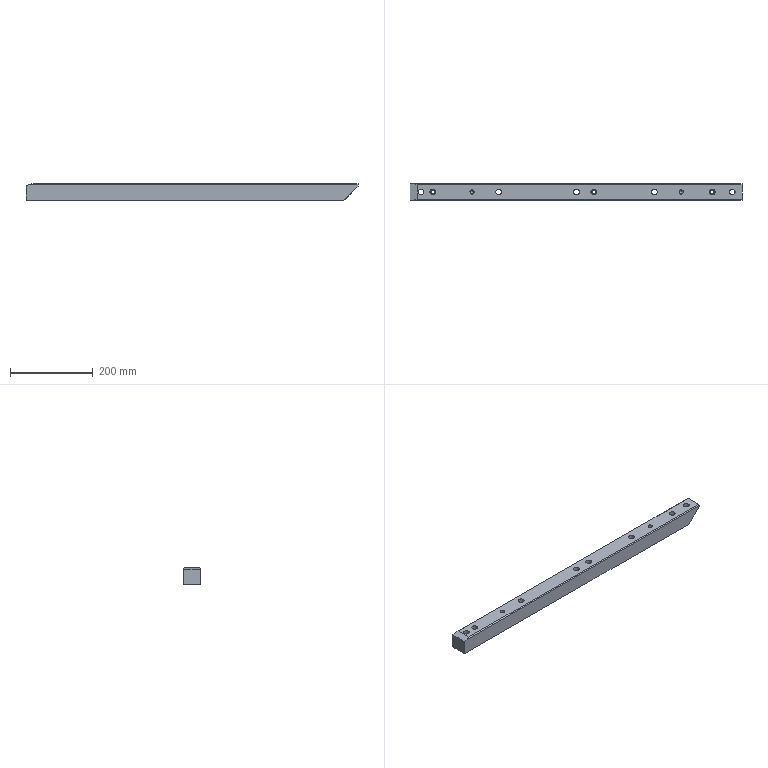Part | NX | features 22 2 | 1 solid | 47 faces | box 802 x 40 x 40 mm | volume 1188494 mm3 | cylinder 24 | plane 19 | cone 4 | commonest cylinder face diameters 14 x8 6 x6 9 x3 25 x3 6.8 x2 10.3 x2
STEP:
#1=CARTESIAN_POINT('',(3434.4,-12.,-43.5));
#2=VERTEX_POINT('',#1);
#3=CARTESIAN_POINT('',(3431.,-12.,-43.5));
#4=DIRECTION('',(0.,0.,1.));
#5=DIRECTION('',(1.,0.,0.));
#6=AXIS2_PLACEMENT_3D('',#3,#4,#5);
#7=CIRCLE('',#6,3.4);
#8=EDGE_CURVE('',#2,#2,#7,.T.);
#9=ORIENTED_EDGE('',*,*,#8,.T.);
#10=EDGE_LOOP('',(#9));
#11=FACE_BOUND('',#10,.T.);
#12=CARTESIAN_POINT('',(3224.306,0.,-43.5));
#13=VERTEX_POINT('',#12);
#14=CARTESIAN_POINT('',(3217.306,0.,-43.5));
#15=DIRECTION('',(0.,0.,-1.));
#16=DIRECTION('',(1.,0.,0.));
#17=AXIS2_PLACEMENT_3D('',#14,#15,#16);
#18=CIRCLE('',#17,7.);
#19=EDGE_CURVE('',#13,#13,#18,.T.);
#20=ORIENTED_EDGE('',*,*,#19,.F.);
#21=EDGE_LOOP('',(#20));
#22=FACE_BOUND('',#21,.T.);
#23=CARTESIAN_POINT('',(2848.306,0.,-43.5));
#24=VERTEX_POINT('',#23);
#25=CARTESIAN_POINT('',(2841.306,0.,-43.5));
#26=DIRECTION('',(0.,0.,-1.));
#27=DIRECTION('',(1.,0.,0.));
#28=AXIS2_PLACEMENT_3D('',#25,#26,#27);
#29=CIRCLE('',#28,7.);
#30=EDGE_CURVE('',#24,#24,#29,.T.);
#31=ORIENTED_EDGE('',*,*,#30,.F.);
#32=EDGE_LOOP('',(#31));
#33=FACE_BOUND('',#32,.T.);
#34=CARTESIAN_POINT('',(3412.306,0.,-43.5));
#35=VERTEX_POINT('',#34);
#36=CARTESIAN_POINT('',(3405.306,0.,-43.5));
#37=DIRECTION('',(0.,0.,-1.));
#38=DIRECTION('',(1.,0.,0.));
#39=AXIS2_PLACEMENT_3D('',#36,#37,#38);
#40=CIRCLE('',#39,7.);
#41=EDGE_CURVE('',#35,#35,#40,.T.);
#42=ORIENTED_EDGE('',*,*,#41,.F.);
#43=EDGE_LOOP('',(#42));
#44=FACE_BOUND('',#43,.T.);
#45=CARTESIAN_POINT('',(3547.701,-11.,-43.5));
#46=VERTEX_POINT('',#45);
#47=CARTESIAN_POINT('',(3542.299,-11.,-43.5));
#48=VERTEX_POINT('',#47);
#49=CARTESIAN_POINT('',(3545.,-11.,-43.5));
#50=DIRECTION('',(-1.,0.,0.));
#51=VECTOR('',#50,1000.);
#52=LINE('',#49,#51);
#53=EDGE_CURVE('',#46,#48,#52,.T.);
#54=ORIENTED_EDGE('',*,*,#53,.F.);
#55=CARTESIAN_POINT('',(3552.847,-9.73,-43.5));
#56=VERTEX_POINT('',#55);
#57=CARTESIAN_POINT('',(3549.937,-9.,-43.5));
#58=DIRECTION('',(0.,0.,-1.));
#59=DIRECTION('',(1.,0.,0.));
#60=AXIS2_PLACEMENT_3D('',#57,#58,#59);
#61=CIRCLE('',#60,3.);
#62=EDGE_CURVE('',#56,#46,#61,.T.);
#63=ORIENTED_EDGE('',*,*,#62,.F.);
#64=CARTESIAN_POINT('',(3537.153,-9.73,-43.5));
#65=VERTEX_POINT('',#64);
#66=CARTESIAN_POINT('',(3545.,0.,-43.5));
#67=DIRECTION('',(0.,0.,-1.));
#68=DIRECTION('',(1.,0.,0.));
#69=AXIS2_PLACEMENT_3D('',#66,#67,#68);
#70=CIRCLE('',#69,12.5);
#71=EDGE_CURVE('',#65,#56,#70,.T.);
#72=ORIENTED_EDGE('',*,*,#71,.F.);
#73=CARTESIAN_POINT('',(3540.063,-9.,-43.5));
#74=DIRECTION('',(0.,0.,-1.));
#75=DIRECTION('',(1.,0.,0.));
#76=AXIS2_PLACEMENT_3D('',#73,#74,#75);
#77=CIRCLE('',#76,3.);
#78=EDGE_CURVE('',#48,#65,#77,.T.);
#79=ORIENTED_EDGE('',*,*,#78,.F.);
#80=EDGE_LOOP('',(#54,#63,#72,#79));
#81=FACE_BOUND('',#80,.T.);
#82=CARTESIAN_POINT('',(2872.701,-11.,-43.5));
#83=VERTEX_POINT('',#82);
#84=CARTESIAN_POINT('',(2867.299,-11.,-43.5));
#85=VERTEX_POINT('',#84);
#86=CARTESIAN_POINT('',(2870.,-11.,-43.5));
#87=DIRECTION('',(-1.,0.,0.));
#88=VECTOR('',#87,1000.);
#89=LINE('',#86,#88);
#90=EDGE_CURVE('',#83,#85,#89,.T.);
#91=ORIENTED_EDGE('',*,*,#90,.F.);
#92=CARTESIAN_POINT('',(2877.847,-9.73,-43.5));
#93=VERTEX_POINT('',#92);
#94=CARTESIAN_POINT('',(2874.937,-9.,-43.5));
#95=DIRECTION('',(0.,0.,-1.));
#96=DIRECTION('',(0.9659,0.2588,0.));
#97=AXIS2_PLACEMENT_3D('',#94,#95,#96);
#98=CIRCLE('',#97,3.);
#99=EDGE_CURVE('',#93,#83,#98,.T.);
#100=ORIENTED_EDGE('',*,*,#99,.F.);
#101=CARTESIAN_POINT('',(2862.153,-9.73,-43.5));
#102=VERTEX_POINT('',#101);
#103=CARTESIAN_POINT('',(2870.,0.,-43.5));
#104=DIRECTION('',(0.,0.,1.));
#105=DIRECTION('',(0.9659,0.2588,0.));
#106=AXIS2_PLACEMENT_3D('',#103,#104,#105);
#107=CIRCLE('',#106,12.5);
#108=EDGE_CURVE('',#93,#102,#107,.T.);
#109=ORIENTED_EDGE('',*,*,#108,.T.);
#110=CARTESIAN_POINT('',(2865.063,-9.,-43.5));
#111=DIRECTION('',(0.,0.,-1.));
#112=DIRECTION('',(0.9659,0.2588,0.));
#113=AXIS2_PLACEMENT_3D('',#110,#111,#112);
#114=CIRCLE('',#113,3.);
#115=EDGE_CURVE('',#85,#102,#114,.T.);
#116=ORIENTED_EDGE('',*,*,#115,.F.);
#117=EDGE_LOOP('',(#91,#100,#109,#116));
#118=FACE_BOUND('',#117,.T.);
#119=CARTESIAN_POINT('',(3583.,20.,-43.5));
#120=VERTEX_POINT('',#119);
#121=CARTESIAN_POINT('',(2815.,20.,-43.5));
#122=VERTEX_POINT('',#121);
#123=CARTESIAN_POINT('',(2860.,20.,-43.5));
#124=DIRECTION('',(-1.,0.,0.));
#125=VECTOR('',#124,1000.);
#126=LINE('',#123,#125);
#127=EDGE_CURVE('',#120,#122,#126,.T.);
#128=ORIENTED_EDGE('',*,*,#127,.F.);
#129=CARTESIAN_POINT('',(3583.,-20.,-43.5));
#130=VERTEX_POINT('',#129);
#131=CARTESIAN_POINT('',(3583.,0.,-43.5));
#132=DIRECTION('',(0.,-1.,0.));
#133=VECTOR('',#132,1000.);
#134=LINE('',#131,#133);
#135=EDGE_CURVE('',#120,#130,#134,.T.);
#136=ORIENTED_EDGE('',*,*,#135,.T.);
#137=CARTESIAN_POINT('',(2815.,-20.,-43.5));
#138=VERTEX_POINT('',#137);
#139=CARTESIAN_POINT('',(2860.,-20.,-43.5));
#140=DIRECTION('',(1.,0.,0.));
#141=VECTOR('',#140,1000.);
#142=LINE('',#139,#141);
#143=EDGE_CURVE('',#138,#130,#142,.T.);
#144=ORIENTED_EDGE('',*,*,#143,.F.);
#145=CARTESIAN_POINT('',(2815.,0.,-43.5));
#146=DIRECTION('',(0.,-1.,0.));
#147=VECTOR('',#146,1000.);
#148=LINE('',#145,#147);
#149=EDGE_CURVE('',#122,#138,#148,.T.);
#150=ORIENTED_EDGE('',*,*,#149,.F.);
#151=EDGE_LOOP('',(#128,#136,#144,#150));
#152=FACE_BOUND('',#151,.T.);
#153=CARTESIAN_POINT('',(3036.306,0.,-43.5));
#154=VERTEX_POINT('',#153);
#155=CARTESIAN_POINT('',(3029.306,0.,-43.5));
#156=DIRECTION('',(0.,0.,-1.));
#157=DIRECTION('',(1.,0.,0.));
#158=AXIS2_PLACEMENT_3D('',#155,#156,#157);
#159=CIRCLE('',#158,7.);
#160=EDGE_CURVE('',#154,#154,#159,.T.);
#161=ORIENTED_EDGE('',*,*,#160,.F.);
#162=EDGE_LOOP('',(#161));
#163=FACE_BOUND('',#162,.T.);
#164=CARTESIAN_POINT('',(3251.153,-9.73,-43.5));
#165=VERTEX_POINT('',#164);
#166=CARTESIAN_POINT('',(3266.847,-9.73,-43.5));
#167=VERTEX_POINT('',#166);
#168=CARTESIAN_POINT('',(3259.,0.,-43.5));
#169=DIRECTION('',(0.,0.,-1.));
#170=DIRECTION('',(1.,0.,0.));
#171=AXIS2_PLACEMENT_3D('',#168,#169,#170);
#172=CIRCLE('',#171,12.5);
#173=EDGE_CURVE('',#165,#167,#172,.T.);
#174=ORIENTED_EDGE('',*,*,#173,.F.);
#175=CARTESIAN_POINT('',(3256.299,-11.,-43.5));
#176=VERTEX_POINT('',#175);
#177=CARTESIAN_POINT('',(3254.063,-9.,-43.5));
#178=DIRECTION('',(0.,0.,1.));
#179=DIRECTION('',(1.,0.,0.));
#180=AXIS2_PLACEMENT_3D('',#177,#178,#179);
#181=CIRCLE('',#180,3.);
#182=EDGE_CURVE('',#165,#176,#181,.T.);
#183=ORIENTED_EDGE('',*,*,#182,.T.);
#184=CARTESIAN_POINT('',(3261.701,-11.,-43.5));
#185=VERTEX_POINT('',#184);
#186=CARTESIAN_POINT('',(2534.879,-11.,-43.5));
#187=DIRECTION('',(1.,0.,0.));
#188=VECTOR('',#187,1000.);
#189=LINE('',#186,#188);
#190=EDGE_CURVE('',#176,#185,#189,.T.);
#191=ORIENTED_EDGE('',*,*,#190,.T.);
#192=CARTESIAN_POINT('',(3263.937,-9.,-43.5));
#193=DIRECTION('',(0.,0.,1.));
#194=DIRECTION('',(1.,0.,0.));
#195=AXIS2_PLACEMENT_3D('',#192,#193,#194);
#196=CIRCLE('',#195,3.);
#197=EDGE_CURVE('',#185,#167,#196,.T.);
#198=ORIENTED_EDGE('',*,*,#197,.T.);
#199=EDGE_LOOP('',(#174,#183,#191,#198));
#200=FACE_BOUND('',#199,.T.);
#201=CARTESIAN_POINT('',(3434.4,12.,-43.5));
#202=VERTEX_POINT('',#201);
#203=CARTESIAN_POINT('',(3431.,12.,-43.5));
#204=DIRECTION('',(0.,0.,1.));
#205=DIRECTION('',(1.,0.,0.));
#206=AXIS2_PLACEMENT_3D('',#203,#204,#205);
#207=CIRCLE('',#206,3.4);
#208=EDGE_CURVE('',#202,#202,#207,.T.);
#209=ORIENTED_EDGE('',*,*,#208,.T.);
#210=EDGE_LOOP('',(#209));
#211=FACE_BOUND('',#210,.T.);
#212=CARTESIAN_POINT('',(2544.879,0.,-43.5));
#213=DIRECTION('',(0.,0.,1.));
#214=DIRECTION('',(-1.,0.,0.));
#215=AXIS2_PLACEMENT_3D('',#212,#213,#214);
#216=PLANE('',#215);
#217=ADVANCED_FACE('',(#11,#22,#33,#44,#81,#118,#152,#163,#200,#211),#216,.F.);
#218=CARTESIAN_POINT('',(3263.229,1.539,-28.5));
#219=VERTEX_POINT('',#218);
#220=CARTESIAN_POINT('',(3259.,0.,-28.5));
#221=DIRECTION('',(0.,0.,1.));
#222=DIRECTION('',(0.9397,0.342,0.));
#223=AXIS2_PLACEMENT_3D('',#220,#221,#222);
#224=CIRCLE('',#223,4.5);
#225=EDGE_CURVE('',#219,#219,#224,.T.);
#226=ORIENTED_EDGE('',*,*,#225,.F.);
#227=EDGE_LOOP('',(#226));
#228=FACE_BOUND('',#227,.T.);
#229=CARTESIAN_POINT('',(3263.5,0.,-15.5));
#230=VERTEX_POINT('',#229);
#231=CARTESIAN_POINT('',(3259.,0.,-15.5));
#232=DIRECTION('',(0.,0.,1.));
#233=DIRECTION('',(1.,0.,0.));
#234=AXIS2_PLACEMENT_3D('',#231,#232,#233);
#235=CIRCLE('',#234,4.5);
#236=EDGE_CURVE('',#230,#230,#235,.T.);
#237=ORIENTED_EDGE('',*,*,#236,.T.);
#238=EDGE_LOOP('',(#237));
#239=FACE_BOUND('',#238,.T.);
#240=CARTESIAN_POINT('',(3259.,0.,49.9));
#241=DIRECTION('',(0.,0.,-1.));
#242=DIRECTION('',(0.342,-0.9397,0.));
#243=AXIS2_PLACEMENT_3D('',#240,#241,#242);
#244=CYLINDRICAL_SURFACE('',#243,4.5);
#245=ADVANCED_FACE('',(#228,#239),#244,.F.);
#246=ORIENTED_EDGE('',*,*,#225,.T.);
#247=EDGE_LOOP('',(#246));
#248=FACE_BOUND('',#247,.T.);
#249=CARTESIAN_POINT('',(3256.299,-11.,-28.5));
#250=VERTEX_POINT('',#249);
#251=CARTESIAN_POINT('',(3251.153,-9.73,-28.5));
#252=VERTEX_POINT('',#251);
#253=CARTESIAN_POINT('',(3254.063,-9.,-28.5));
#254=DIRECTION('',(0.,0.,-1.));
#255=DIRECTION('',(0.9397,-0.342,0.));
#256=AXIS2_PLACEMENT_3D('',#253,#254,#255);
#257=CIRCLE('',#256,3.);
#258=EDGE_CURVE('',#250,#252,#257,.T.);
#259=ORIENTED_EDGE('',*,*,#258,.T.);
#260=CARTESIAN_POINT('',(3266.847,-9.73,-28.5));
#261=VERTEX_POINT('',#260);
#262=CARTESIAN_POINT('',(3259.,0.,-28.5));
#263=DIRECTION('',(0.,0.,-1.));
#264=DIRECTION('',(0.,1.,0.));
#265=AXIS2_PLACEMENT_3D('',#262,#263,#264);
#266=CIRCLE('',#265,12.5);
#267=EDGE_CURVE('',#252,#261,#266,.T.);
#268=ORIENTED_EDGE('',*,*,#267,.T.);
#269=CARTESIAN_POINT('',(3261.701,-11.,-28.5));
#270=VERTEX_POINT('',#269);
#271=CARTESIAN_POINT('',(3263.937,-9.,-28.5));
#272=DIRECTION('',(0.,0.,1.));
#273=DIRECTION('',(-0.9397,-0.342,0.));
#274=AXIS2_PLACEMENT_3D('',#271,#272,#273);
#275=CIRCLE('',#274,3.);
#276=EDGE_CURVE('',#270,#261,#275,.T.);
#277=ORIENTED_EDGE('',*,*,#276,.F.);
#278=CARTESIAN_POINT('',(3259.,-11.,-28.5));
#279=DIRECTION('',(-1.,0.,0.));
#280=VECTOR('',#279,1000.);
#281=LINE('',#278,#280);
#282=EDGE_CURVE('',#270,#250,#281,.T.);
#283=ORIENTED_EDGE('',*,*,#282,.T.);
#284=EDGE_LOOP('',(#259,#268,#277,#283));
#285=FACE_BOUND('',#284,.T.);
#286=CARTESIAN_POINT('',(3259.,0.,-28.5));
#287=DIRECTION('',(0.,0.,1.));
#288=DIRECTION('',(0.,-1.,0.));
#289=AXIS2_PLACEMENT_3D('',#286,#287,#288);
#290=PLANE('',#289);
#291=ADVANCED_FACE('',(#248,#285),#290,.F.);
#292=ORIENTED_EDGE('',*,*,#282,.F.);
#293=CARTESIAN_POINT('',(3261.701,-11.,-41.5));
#294=DIRECTION('',(0.,0.,1.));
#295=VECTOR('',#294,1000.);
#296=LINE('',#293,#295);
#297=EDGE_CURVE('',#185,#270,#296,.T.);
#298=ORIENTED_EDGE('',*,*,#297,.F.);
#299=ORIENTED_EDGE('',*,*,#190,.F.);
#300=CARTESIAN_POINT('',(3256.299,-11.,-41.5));
#301=DIRECTION('',(0.,0.,1.));
#302=VECTOR('',#301,1000.);
#303=LINE('',#300,#302);
#304=EDGE_CURVE('',#176,#250,#303,.T.);
#305=ORIENTED_EDGE('',*,*,#304,.T.);
#306=EDGE_LOOP('',(#292,#298,#299,#305));
#307=FACE_BOUND('',#306,.T.);
#308=CARTESIAN_POINT('',(3259.,-11.,-126.5));
#309=DIRECTION('',(0.,1.,0.));
#310=DIRECTION('',(0.,0.,-1.));
#311=AXIS2_PLACEMENT_3D('',#308,#309,#310);
#312=PLANE('',#311);
#313=ADVANCED_FACE('',(#307),#312,.T.);
#314=CARTESIAN_POINT('',(3266.847,-9.73,-34.));
#315=DIRECTION('',(0.,0.,-1.));
#316=VECTOR('',#315,1000.);
#317=LINE('',#314,#316);
#318=EDGE_CURVE('',#261,#167,#317,.T.);
#319=ORIENTED_EDGE('',*,*,#318,.F.);
#320=ORIENTED_EDGE('',*,*,#267,.F.);
#321=CARTESIAN_POINT('',(3251.153,-9.73,-34.));
#322=DIRECTION('',(0.,0.,-1.));
#323=VECTOR('',#322,1000.);
#324=LINE('',#321,#323);
#325=EDGE_CURVE('',#252,#165,#324,.T.);
#326=ORIENTED_EDGE('',*,*,#325,.T.);
#327=ORIENTED_EDGE('',*,*,#173,.T.);
#328=EDGE_LOOP('',(#319,#320,#326,#327));
#329=FACE_BOUND('',#328,.T.);
#330=CARTESIAN_POINT('',(3259.,0.,-96.5));
#331=DIRECTION('',(0.,0.,-1.));
#332=DIRECTION('',(0.,1.,0.));
#333=AXIS2_PLACEMENT_3D('',#330,#331,#332);
#334=CYLINDRICAL_SURFACE('',#333,12.5);
#335=ADVANCED_FACE('',(#329),#334,.F.);
#336=ORIENTED_EDGE('',*,*,#318,.T.);
#337=ORIENTED_EDGE('',*,*,#197,.F.);
#338=ORIENTED_EDGE('',*,*,#297,.T.);
#339=ORIENTED_EDGE('',*,*,#276,.T.);
#340=EDGE_LOOP('',(#336,#337,#338,#339));
#341=FACE_BOUND('',#340,.T.);
#342=CARTESIAN_POINT('',(3263.937,-9.,-41.5));
#343=DIRECTION('',(0.,0.,1.));
#344=DIRECTION('',(-0.9397,-0.342,0.));
#345=AXIS2_PLACEMENT_3D('',#342,#343,#344);
#346=CYLINDRICAL_SURFACE('',#345,3.);
#347=ADVANCED_FACE('',(#341),#346,.F.);
#348=ORIENTED_EDGE('',*,*,#325,.F.);
#349=ORIENTED_EDGE('',*,*,#258,.F.);
#350=ORIENTED_EDGE('',*,*,#304,.F.);
#351=ORIENTED_EDGE('',*,*,#182,.F.);
#352=EDGE_LOOP('',(#348,#349,#350,#351));
#353=FACE_BOUND('',#352,.T.);
#354=CARTESIAN_POINT('',(3254.063,-9.,-41.5));
#355=DIRECTION('',(0.,0.,1.));
#356=DIRECTION('',(0.9397,-0.342,0.));
#357=AXIS2_PLACEMENT_3D('',#354,#355,#356);
#358=CYLINDRICAL_SURFACE('',#357,3.);
#359=ADVANCED_FACE('',(#353),#358,.F.);
#360=CARTESIAN_POINT('',(3266.,0.,-15.5));
#361=VERTEX_POINT('',#360);
#362=CARTESIAN_POINT('',(3259.,0.,-15.5));
#363=DIRECTION('',(0.,0.,1.));
#364=DIRECTION('',(1.,0.,0.));
#365=AXIS2_PLACEMENT_3D('',#362,#363,#364);
#366=CIRCLE('',#365,7.);
#367=EDGE_CURVE('',#361,#361,#366,.T.);
#368=ORIENTED_EDGE('',*,*,#367,.T.);
#369=EDGE_LOOP('',(#368));
#370=FACE_BOUND('',#369,.T.);
#371=ORIENTED_EDGE('',*,*,#236,.F.);
#372=EDGE_LOOP('',(#371));
#373=FACE_BOUND('',#372,.T.);
#374=CARTESIAN_POINT('',(3377.182,268.173,-15.5));
#375=DIRECTION('',(0.,0.,1.));
#376=DIRECTION('',(-0.9397,-0.342,0.));
#377=AXIS2_PLACEMENT_3D('',#374,#375,#376);
#378=PLANE('',#377);
#379=ADVANCED_FACE('',(#370,#373),#378,.T.);
#380=CARTESIAN_POINT('',(3266.,0.,-3.5));
#381=VERTEX_POINT('',#380);
#382=CARTESIAN_POINT('',(3259.,0.,-3.5));
#383=DIRECTION('',(0.,0.,1.));
#384=DIRECTION('',(1.,0.,0.));
#385=AXIS2_PLACEMENT_3D('',#382,#383,#384);
#386=CIRCLE('',#385,7.);
#387=EDGE_CURVE('',#381,#381,#386,.T.);
#388=ORIENTED_EDGE('',*,*,#387,.T.);
#389=EDGE_LOOP('',(#388));
#390=FACE_BOUND('',#389,.T.);
#391=ORIENTED_EDGE('',*,*,#367,.F.);
#392=EDGE_LOOP('',(#391));
#393=FACE_BOUND('',#392,.T.);
#394=CARTESIAN_POINT('',(3259.,0.,-9.5));
#395=DIRECTION('',(0.,0.,1.));
#396=DIRECTION('',(-0.9397,-0.342,0.));
#397=AXIS2_PLACEMENT_3D('',#394,#395,#396);
#398=CYLINDRICAL_SURFACE('',#397,7.);
#399=ADVANCED_FACE('',(#390,#393),#398,.F.);
#400=CARTESIAN_POINT('',(2874.229,1.539,-28.5));
#401=VERTEX_POINT('',#400);
#402=CARTESIAN_POINT('',(2870.,0.,-28.5));
#403=DIRECTION('',(0.,0.,1.));
#404=DIRECTION('',(0.9397,0.342,0.));
#405=AXIS2_PLACEMENT_3D('',#402,#403,#404);
#406=CIRCLE('',#405,4.5);
#407=EDGE_CURVE('',#401,#401,#406,.T.);
#408=ORIENTED_EDGE('',*,*,#407,.F.);
#409=EDGE_LOOP('',(#408));
#410=FACE_BOUND('',#409,.T.);
#411=CARTESIAN_POINT('',(2874.5,0.,-15.5));
#412=VERTEX_POINT('',#411);
#413=CARTESIAN_POINT('',(2870.,0.,-15.5));
#414=DIRECTION('',(0.,0.,1.));
#415=DIRECTION('',(1.,0.,0.));
#416=AXIS2_PLACEMENT_3D('',#413,#414,#415);
#417=CIRCLE('',#416,4.5);
#418=EDGE_CURVE('',#412,#412,#417,.T.);
#419=ORIENTED_EDGE('',*,*,#418,.T.);
#420=EDGE_LOOP('',(#419));
#421=FACE_BOUND('',#420,.T.);
#422=CARTESIAN_POINT('',(2870.,0.,49.9));
#423=DIRECTION('',(0.,0.,-1.));
#424=DIRECTION('',(0.342,-0.9397,0.));
#425=AXIS2_PLACEMENT_3D('',#422,#423,#424);
#426=CYLINDRICAL_SURFACE('',#425,4.5);
#427=ADVANCED_FACE('',(#410,#421),#426,.F.);
#428=CARTESIAN_POINT('',(3545.,-4.5,-28.5));
#429=VERTEX_POINT('',#428);
#430=CARTESIAN_POINT('',(3545.,0.,-28.5));
#431=DIRECTION('',(0.,0.,1.));
#432=DIRECTION('',(0.,-1.,0.));
#433=AXIS2_PLACEMENT_3D('',#430,#431,#432);
#434=CIRCLE('',#433,4.5);
#435=EDGE_CURVE('',#429,#429,#434,.T.);
#436=ORIENTED_EDGE('',*,*,#435,.F.);
#437=EDGE_LOOP('',(#436));
#438=FACE_BOUND('',#437,.T.);
#439=CARTESIAN_POINT('',(3545.,-4.5,-15.5));
#440=VERTEX_POINT('',#439);
#441=CARTESIAN_POINT('',(3545.,0.,-15.5));
#442=DIRECTION('',(0.,0.,1.));
#443=DIRECTION('',(0.,-1.,0.));
#444=AXIS2_PLACEMENT_3D('',#441,#442,#443);
#445=CIRCLE('',#444,4.5);
#446=EDGE_CURVE('',#440,#440,#445,.T.);
#447=ORIENTED_EDGE('',*,*,#446,.T.);
#448=EDGE_LOOP('',(#447));
#449=FACE_BOUND('',#448,.T.);
#450=CARTESIAN_POINT('',(3545.,0.,49.9));
#451=DIRECTION('',(0.,0.,-1.));
#452=DIRECTION('',(0.342,-0.9397,0.));
#453=AXIS2_PLACEMENT_3D('',#450,#451,#452);
#454=CYLINDRICAL_SURFACE('',#453,4.5);
#455=ADVANCED_FACE('',(#438,#449),#454,.F.);
#456=CARTESIAN_POINT('',(2965.,0.,-42.5));
#457=VERTEX_POINT('',#456);
#458=VERTEX_LOOP('',#457);
#459=FACE_BOUND('',#458,.T.);
#460=CARTESIAN_POINT('',(2959.85,0.,-37.35));
#461=VERTEX_POINT('',#460);
#462=CARTESIAN_POINT('',(2965.,0.,-37.35));
#463=DIRECTION('',(0.,0.,-1.));
#464=DIRECTION('',(-1.,0.,0.));
#465=AXIS2_PLACEMENT_3D('',#462,#463,#464);
#466=CIRCLE('',#465,5.15);
#467=EDGE_CURVE('',#461,#461,#466,.T.);
#468=ORIENTED_EDGE('',*,*,#467,.F.);
#469=EDGE_LOOP('',(#468));
#470=FACE_BOUND('',#469,.T.);
#471=CARTESIAN_POINT('',(2965.,0.,-37.35));
#472=DIRECTION('',(0.,0.,1.));
#473=DIRECTION('',(-1.,0.,0.));
#474=AXIS2_PLACEMENT_3D('',#471,#472,#473);
#475=CONICAL_SURFACE('',#474,5.15,0.7854);
#476=ADVANCED_FACE('',(#459,#470),#475,.F.);
#477=CARTESIAN_POINT('',(2877.,0.,-15.5));
#478=VERTEX_POINT('',#477);
#479=CARTESIAN_POINT('',(2870.,0.,-15.5));
#480=DIRECTION('',(0.,0.,1.));
#481=DIRECTION('',(1.,0.,0.));
#482=AXIS2_PLACEMENT_3D('',#479,#480,#481);
#483=CIRCLE('',#482,7.);
#484=EDGE_CURVE('',#478,#478,#483,.T.);
#485=ORIENTED_EDGE('',*,*,#484,.T.);
#486=EDGE_LOOP('',(#485));
#487=FACE_BOUND('',#486,.T.);
#488=ORIENTED_EDGE('',*,*,#418,.F.);
#489=EDGE_LOOP('',(#488));
#490=FACE_BOUND('',#489,.T.);
#491=CARTESIAN_POINT('',(2978.182,268.173,-15.5));
#492=DIRECTION('',(0.,0.,1.));
#493=DIRECTION('',(-0.9397,-0.342,0.));
#494=AXIS2_PLACEMENT_3D('',#491,#492,#493);
#495=PLANE('',#494);
#496=ADVANCED_FACE('',(#487,#490),#495,.T.);
#497=CARTESIAN_POINT('',(3545.,-7.,-15.5));
#498=VERTEX_POINT('',#497);
#499=CARTESIAN_POINT('',(3545.,0.,-15.5));
#500=DIRECTION('',(0.,0.,1.));
#501=DIRECTION('',(0.,-1.,0.));
#502=AXIS2_PLACEMENT_3D('',#499,#500,#501);
#503=CIRCLE('',#502,7.);
#504=EDGE_CURVE('',#498,#498,#503,.T.);
#505=ORIENTED_EDGE('',*,*,#504,.T.);
#506=EDGE_LOOP('',(#505));
#507=FACE_BOUND('',#506,.T.);
#508=ORIENTED_EDGE('',*,*,#446,.F.);
#509=EDGE_LOOP('',(#508));
#510=FACE_BOUND('',#509,.T.);
#511=CARTESIAN_POINT('',(3653.182,268.173,-15.5));
#512=DIRECTION('',(0.,0.,1.));
#513=DIRECTION('',(-0.9397,-0.342,0.));
#514=AXIS2_PLACEMENT_3D('',#511,#512,#513);
#515=PLANE('',#514);
#516=ADVANCED_FACE('',(#507,#510),#515,.T.);
#517=CARTESIAN_POINT('',(3470.,0.,-42.5));
#518=VERTEX_POINT('',#517);
#519=VERTEX_LOOP('',#518);
#520=FACE_BOUND('',#519,.T.);
#521=CARTESIAN_POINT('',(3464.85,0.,-37.35));
#522=VERTEX_POINT('',#521);
#523=CARTESIAN_POINT('',(3470.,0.,-37.35));
#524=DIRECTION('',(0.,0.,-1.));
#525=DIRECTION('',(-1.,0.,0.));
#526=AXIS2_PLACEMENT_3D('',#523,#524,#525);
#527=CIRCLE('',#526,5.15);
#528=EDGE_CURVE('',#522,#522,#527,.T.);
#529=ORIENTED_EDGE('',*,*,#528,.F.);
#530=EDGE_LOOP('',(#529));
#531=FACE_BOUND('',#530,.T.);
#532=CARTESIAN_POINT('',(3470.,0.,-37.35));
#533=DIRECTION('',(0.,0.,1.));
#534=DIRECTION('',(-1.,0.,0.));
#535=AXIS2_PLACEMENT_3D('',#532,#533,#534);
#536=CONICAL_SURFACE('',#535,5.15,0.7854);
#537=ADVANCED_FACE('',(#520,#531),#536,.F.);
#538=ORIENTED_EDGE('',*,*,#407,.T.);
#539=EDGE_LOOP('',(#538));
#540=FACE_BOUND('',#539,.T.);
#541=CARTESIAN_POINT('',(2867.299,-11.,-28.5));
#542=VERTEX_POINT('',#541);
#543=CARTESIAN_POINT('',(2862.153,-9.73,-28.5));
#544=VERTEX_POINT('',#543);
#545=CARTESIAN_POINT('',(2865.063,-9.,-28.5));
#546=DIRECTION('',(0.,0.,-1.));
#547=DIRECTION('',(0.9397,-0.342,0.));
#548=AXIS2_PLACEMENT_3D('',#545,#546,#547);
#549=CIRCLE('',#548,3.);
#550=EDGE_CURVE('',#542,#544,#549,.T.);
#551=ORIENTED_EDGE('',*,*,#550,.T.);
#552=CARTESIAN_POINT('',(2877.847,-9.73,-28.5));
#553=VERTEX_POINT('',#552);
#554=CARTESIAN_POINT('',(2870.,0.,-28.5));
#555=DIRECTION('',(0.,0.,-1.));
#556=DIRECTION('',(0.,1.,0.));
#557=AXIS2_PLACEMENT_3D('',#554,#555,#556);
#558=CIRCLE('',#557,12.5);
#559=EDGE_CURVE('',#544,#553,#558,.T.);
#560=ORIENTED_EDGE('',*,*,#559,.T.);
#561=CARTESIAN_POINT('',(2872.701,-11.,-28.5));
#562=VERTEX_POINT('',#561);
#563=CARTESIAN_POINT('',(2874.937,-9.,-28.5));
#564=DIRECTION('',(0.,0.,1.));
#565=DIRECTION('',(-0.9397,-0.342,0.));
#566=AXIS2_PLACEMENT_3D('',#563,#564,#565);
#567=CIRCLE('',#566,3.);
#568=EDGE_CURVE('',#562,#553,#567,.T.);
#569=ORIENTED_EDGE('',*,*,#568,.F.);
#570=CARTESIAN_POINT('',(2870.,-11.,-28.5));
#571=DIRECTION('',(-1.,0.,0.));
#572=VECTOR('',#571,1000.);
#573=LINE('',#570,#572);
#574=EDGE_CURVE('',#562,#542,#573,.T.);
#575=ORIENTED_EDGE('',*,*,#574,.T.);
#576=EDGE_LOOP('',(#551,#560,#569,#575));
#577=FACE_BOUND('',#576,.T.);
#578=CARTESIAN_POINT('',(2870.,0.,-28.5));
#579=DIRECTION('',(0.,0.,1.));
#580=DIRECTION('',(0.,-1.,0.));
#581=AXIS2_PLACEMENT_3D('',#578,#579,#580);
#582=PLANE('',#581);
#583=ADVANCED_FACE('',(#540,#577),#582,.F.);
#584=ORIENTED_EDGE('',*,*,#435,.T.);
#585=EDGE_LOOP('',(#584));
#586=FACE_BOUND('',#585,.T.);
#587=CARTESIAN_POINT('',(3542.299,-11.,-28.5));
#588=VERTEX_POINT('',#587);
#589=CARTESIAN_POINT('',(3537.153,-9.73,-28.5));
#590=VERTEX_POINT('',#589);
#591=CARTESIAN_POINT('',(3540.063,-9.,-28.5));
#592=DIRECTION('',(0.,0.,-1.));
#593=DIRECTION('',(0.,-1.,0.));
#594=AXIS2_PLACEMENT_3D('',#591,#592,#593);
#595=CIRCLE('',#594,3.);
#596=EDGE_CURVE('',#588,#590,#595,.T.);
#597=ORIENTED_EDGE('',*,*,#596,.T.);
#598=CARTESIAN_POINT('',(3552.847,-9.73,-28.5));
#599=VERTEX_POINT('',#598);
#600=CARTESIAN_POINT('',(3545.,0.,-28.5));
#601=DIRECTION('',(0.,0.,-1.));
#602=DIRECTION('',(0.,-1.,0.));
#603=AXIS2_PLACEMENT_3D('',#600,#601,#602);
#604=CIRCLE('',#603,12.5);
#605=EDGE_CURVE('',#590,#599,#604,.T.);
#606=ORIENTED_EDGE('',*,*,#605,.T.);
#607=CARTESIAN_POINT('',(3547.701,-11.,-28.5));
#608=VERTEX_POINT('',#607);
#609=CARTESIAN_POINT('',(3549.937,-9.,-28.5));
#610=DIRECTION('',(0.,0.,1.));
#611=DIRECTION('',(0.,-1.,0.));
#612=AXIS2_PLACEMENT_3D('',#609,#610,#611);
#613=CIRCLE('',#612,3.);
#614=EDGE_CURVE('',#608,#599,#613,.T.);
#615=ORIENTED_EDGE('',*,*,#614,.F.);
#616=CARTESIAN_POINT('',(3545.,-11.,-28.5));
#617=DIRECTION('',(-1.,0.,0.));
#618=VECTOR('',#617,1000.);
#619=LINE('',#616,#618);
#620=EDGE_CURVE('',#608,#588,#619,.T.);
#621=ORIENTED_EDGE('',*,*,#620,.T.);
#622=EDGE_LOOP('',(#597,#606,#615,#621));
#623=FACE_BOUND('',#622,.T.);
#624=CARTESIAN_POINT('',(3545.,0.,-28.5));
#625=DIRECTION('',(0.,0.,1.));
#626=DIRECTION('',(0.,-1.,0.));
#627=AXIS2_PLACEMENT_3D('',#624,#625,#626);
#628=PLANE('',#627);
#629=ADVANCED_FACE('',(#586,#623),#628,.F.);
#630=ORIENTED_EDGE('',*,*,#467,.T.);
#631=EDGE_LOOP('',(#630));
#632=FACE_BOUND('',#631,.T.);
#633=CARTESIAN_POINT('',(2970.15,0.,-3.5));
#634=VERTEX_POINT('',#633);
#635=CARTESIAN_POINT('',(2965.,0.,-3.5));
#636=DIRECTION('',(0.,0.,-1.));
#637=DIRECTION('',(1.,0.,0.));
#638=AXIS2_PLACEMENT_3D('',#635,#636,#637);
#639=CIRCLE('',#638,5.15);
#640=EDGE_CURVE('',#634,#634,#639,.T.);
#641=ORIENTED_EDGE('',*,*,#640,.F.);
#642=EDGE_LOOP('',(#641));
#643=FACE_BOUND('',#642,.T.);
#644=CARTESIAN_POINT('',(2965.,0.,-3.5));
#645=DIRECTION('',(0.,0.,-1.));
#646=DIRECTION('',(-1.,0.,0.));
#647=AXIS2_PLACEMENT_3D('',#644,#645,#646);
#648=CYLINDRICAL_SURFACE('',#647,5.15);
#649=ADVANCED_FACE('',(#632,#643),#648,.F.);
#650=CARTESIAN_POINT('',(3600.306,0.,-3.5));
#651=VERTEX_POINT('',#650);
#652=CARTESIAN_POINT('',(3593.306,0.,-3.5));
#653=DIRECTION('',(0.,0.,-1.));
#654=DIRECTION('',(1.,0.,0.));
#655=AXIS2_PLACEMENT_3D('',#652,#653,#654);
#656=CIRCLE('',#655,7.);
#657=EDGE_CURVE('',#651,#651,#656,.T.);
#658=ORIENTED_EDGE('',*,*,#657,.F.);
#659=EDGE_LOOP('',(#658));
#660=FACE_BOUND('',#659,.T.);
#661=CARTESIAN_POINT('',(3600.306,0.,-26.194));
#662=VERTEX_POINT('',#661);
#663=CARTESIAN_POINT('',(3593.306,0.,-33.194));
#664=DIRECTION('',(0.7071,0.,-0.7071));
#665=DIRECTION('',(0.7071,0.,0.7071));
#666=AXIS2_PLACEMENT_3D('',#663,#664,#665);
#667=ELLIPSE('',#666,9.899,7.);
#668=EDGE_CURVE('',#662,#662,#667,.T.);
#669=ORIENTED_EDGE('',*,*,#668,.T.);
#670=EDGE_LOOP('',(#669));
#671=FACE_BOUND('',#670,.T.);
#672=CARTESIAN_POINT('',(3593.306,0.,-87.));
#673=DIRECTION('',(0.,0.,1.));
#674=DIRECTION('',(-1.,0.,0.));
#675=AXIS2_PLACEMENT_3D('',#672,#673,#674);
#676=CYLINDRICAL_SURFACE('',#675,7.);
#677=ADVANCED_FACE('',(#660,#671),#676,.F.);
#678=CARTESIAN_POINT('',(2815.,-20.,-7.75));
#679=VERTEX_POINT('',#678);
#680=CARTESIAN_POINT('',(2815.,20.,-7.75));
#681=VERTEX_POINT('',#680);
#682=CARTESIAN_POINT('',(2815.,0.,-7.75));
#683=DIRECTION('',(0.,1.,0.));
#684=VECTOR('',#683,1000.);
#685=LINE('',#682,#684);
#686=EDGE_CURVE('',#679,#681,#685,.T.);
#687=ORIENTED_EDGE('',*,*,#686,.F.);
#688=CARTESIAN_POINT('',(2824.,-20.,-5.5));
#689=VERTEX_POINT('',#688);
#690=CARTESIAN_POINT('',(2812.,-20.,-8.5));
#691=DIRECTION('',(-0.9701,0.,-0.2425));
#692=VECTOR('',#691,1000.);
#693=LINE('',#690,#692);
#694=EDGE_CURVE('',#689,#679,#693,.T.);
#695=ORIENTED_EDGE('',*,*,#694,.F.);
#696=CARTESIAN_POINT('',(2832.,-18.,-3.5));
#697=VERTEX_POINT('',#696);
#698=CARTESIAN_POINT('',(2817.111,-21.722,-7.222));
#699=DIRECTION('',(-0.9428,-0.2357,-0.2357));
#700=VECTOR('',#699,1000.);
#701=LINE('',#698,#700);
#702=EDGE_CURVE('',#697,#689,#701,.T.);
#703=ORIENTED_EDGE('',*,*,#702,.F.);
#704=CARTESIAN_POINT('',(2832.,18.,-3.5));
#705=VERTEX_POINT('',#704);
#706=CARTESIAN_POINT('',(2832.,0.,-3.5));
#707=DIRECTION('',(0.,-1.,0.));
#708=VECTOR('',#707,1000.);
#709=LINE('',#706,#708);
#710=EDGE_CURVE('',#705,#697,#709,.T.);
#711=ORIENTED_EDGE('',*,*,#710,.F.);
#712=CARTESIAN_POINT('',(2824.,20.,-5.5));
#713=VERTEX_POINT('',#712);
#714=CARTESIAN_POINT('',(2817.111,21.722,-7.222));
#715=DIRECTION('',(0.9428,-0.2357,0.2357));
#716=VECTOR('',#715,1000.);
#717=LINE('',#714,#716);
#718=EDGE_CURVE('',#713,#705,#717,.T.);
#719=ORIENTED_EDGE('',*,*,#718,.F.);
#720=CARTESIAN_POINT('',(2812.,20.,-8.5));
#721=DIRECTION('',(0.9701,0.,0.2425));
#722=VECTOR('',#721,1000.);
#723=LINE('',#720,#722);
#724=EDGE_CURVE('',#681,#713,#723,.T.);
#725=ORIENTED_EDGE('',*,*,#724,.F.);
#726=EDGE_LOOP('',(#687,#695,#703,#711,#719,#725));
#727=FACE_BOUND('',#726,.T.);
#728=CARTESIAN_POINT('',(2812.,0.,-8.5));
#729=DIRECTION('',(0.2425,0.,-0.9701));
#730=DIRECTION('',(0.,-1.,0.));
#731=AXIS2_PLACEMENT_3D('',#728,#729,#730);
#732=PLANE('',#731);
#733=ADVANCED_FACE('',(#727),#732,.F.);
#734=CARTESIAN_POINT('',(3617.,18.,-3.5));
#735=VERTEX_POINT('',#734);
#736=CARTESIAN_POINT('',(2544.879,18.,-3.5));
#737=DIRECTION('',(-1.,0.,0.));
#738=VECTOR('',#737,1000.);
#739=LINE('',#736,#738);
#740=EDGE_CURVE('',#735,#705,#739,.T.);
#741=ORIENTED_EDGE('',*,*,#740,.F.);
#742=CARTESIAN_POINT('',(3617.,20.,-5.5));
#743=VERTEX_POINT('',#742);
#744=CARTESIAN_POINT('',(3617.,18.,-3.5));
#745=DIRECTION('',(0.,0.7071,-0.7071));
#746=VECTOR('',#745,1000.);
#747=LINE('',#744,#746);
#748=EDGE_CURVE('',#735,#743,#747,.T.);
#749=ORIENTED_EDGE('',*,*,#748,.T.);
#750=CARTESIAN_POINT('',(2860.,20.,-5.5));
#751=DIRECTION('',(1.,0.,0.));
#752=VECTOR('',#751,1000.);
#753=LINE('',#750,#752);
#754=EDGE_CURVE('',#713,#743,#753,.T.);
#755=ORIENTED_EDGE('',*,*,#754,.F.);
#756=ORIENTED_EDGE('',*,*,#718,.T.);
#757=EDGE_LOOP('',(#741,#749,#755,#756));
#758=FACE_BOUND('',#757,.T.);
#759=CARTESIAN_POINT('',(2544.879,18.,-3.5));
#760=DIRECTION('',(0.,-0.7071,-0.7071));
#761=DIRECTION('',(0.,-0.7071,0.7071));
#762=AXIS2_PLACEMENT_3D('',#759,#760,#761);
#763=PLANE('',#762);
#764=ADVANCED_FACE('',(#758),#763,.F.);
#765=ORIENTED_EDGE('',*,*,#748,.F.);
#766=CARTESIAN_POINT('',(3617.,-18.,-3.5));
#767=VERTEX_POINT('',#766);
#768=CARTESIAN_POINT('',(3617.,0.,-3.5));
#769=DIRECTION('',(0.,1.,0.));
#770=VECTOR('',#769,1000.);
#771=LINE('',#768,#770);
#772=EDGE_CURVE('',#767,#735,#771,.T.);
#773=ORIENTED_EDGE('',*,*,#772,.F.);
#774=CARTESIAN_POINT('',(3617.,-20.,-5.5));
#775=VERTEX_POINT('',#774);
#776=CARTESIAN_POINT('',(3617.,-18.,-3.5));
#777=DIRECTION('',(0.,0.7071,0.7071));
#778=VECTOR('',#777,1000.);
#779=LINE('',#776,#778);
#780=EDGE_CURVE('',#775,#767,#779,.T.);
#781=ORIENTED_EDGE('',*,*,#780,.F.);
#782=CARTESIAN_POINT('',(3617.,-20.,-9.5));
#783=VERTEX_POINT('',#782);
#784=CARTESIAN_POINT('',(3617.,-20.,-23.5));
#785=DIRECTION('',(0.,0.,1.));
#786=VECTOR('',#785,1000.);
#787=LINE('',#784,#786);
#788=EDGE_CURVE('',#783,#775,#787,.T.);
#789=ORIENTED_EDGE('',*,*,#788,.F.);
#790=CARTESIAN_POINT('',(3617.,20.,-9.5));
#791=VERTEX_POINT('',#790);
#792=CARTESIAN_POINT('',(3617.,0.,-9.5));
#793=DIRECTION('',(0.,-1.,0.));
#794=VECTOR('',#793,1000.);
#795=LINE('',#792,#794);
#796=EDGE_CURVE('',#791,#783,#795,.T.);
#797=ORIENTED_EDGE('',*,*,#796,.F.);
#798=CARTESIAN_POINT('',(3617.,20.,-23.5));
#799=DIRECTION('',(0.,0.,-1.));
#800=VECTOR('',#799,1000.);
#801=LINE('',#798,#800);
#802=EDGE_CURVE('',#743,#791,#801,.T.);
#803=ORIENTED_EDGE('',*,*,#802,.F.);
#804=EDGE_LOOP('',(#765,#773,#781,#789,#797,#803));
#805=FACE_BOUND('',#804,.T.);
#806=CARTESIAN_POINT('',(3617.,-58.,0.));
#807=DIRECTION('',(1.,0.,0.));
#808=DIRECTION('',(0.,0.,1.));
#809=AXIS2_PLACEMENT_3D('',#806,#807,#808);
#810=PLANE('',#809);
#811=ADVANCED_FACE('',(#805),#810,.T.);
#812=CARTESIAN_POINT('',(2860.,-20.,-5.5));
#813=DIRECTION('',(-1.,0.,0.));
#814=VECTOR('',#813,1000.);
#815=LINE('',#812,#814);
#816=EDGE_CURVE('',#775,#689,#815,.T.);
#817=ORIENTED_EDGE('',*,*,#816,.F.);
#818=ORIENTED_EDGE('',*,*,#780,.T.);
#819=CARTESIAN_POINT('',(2544.879,-18.,-3.5));
#820=DIRECTION('',(1.,0.,0.));
#821=VECTOR('',#820,1000.);
#822=LINE('',#819,#821);
#823=EDGE_CURVE('',#697,#767,#822,.T.);
#824=ORIENTED_EDGE('',*,*,#823,.F.);
#825=ORIENTED_EDGE('',*,*,#702,.T.);
#826=EDGE_LOOP('',(#817,#818,#824,#825));
#827=FACE_BOUND('',#826,.T.);
#828=CARTESIAN_POINT('',(2544.879,-18.,-3.5));
#829=DIRECTION('',(0.,0.7071,-0.7071));
#830=DIRECTION('',(0.,-0.7071,-0.7071));
#831=AXIS2_PLACEMENT_3D('',#828,#829,#830);
#832=PLANE('',#831);
#833=ADVANCED_FACE('',(#827),#832,.F.);
#834=CARTESIAN_POINT('',(2876.578,2.394,-3.5));
#835=VERTEX_POINT('',#834);
#836=CARTESIAN_POINT('',(2870.,0.,-3.5));
#837=DIRECTION('',(0.,0.,-1.));
#838=DIRECTION('',(0.9397,0.342,0.));
#839=AXIS2_PLACEMENT_3D('',#836,#837,#838);
#840=CIRCLE('',#839,7.);
#841=EDGE_CURVE('',#835,#835,#840,.T.);
#842=ORIENTED_EDGE('',*,*,#841,.F.);
#843=EDGE_LOOP('',(#842));
#844=FACE_BOUND('',#843,.T.);
#845=ORIENTED_EDGE('',*,*,#484,.F.);
#846=EDGE_LOOP('',(#845));
#847=FACE_BOUND('',#846,.T.);
#848=CARTESIAN_POINT('',(2870.,0.,-9.5));
#849=DIRECTION('',(0.,0.,1.));
#850=DIRECTION('',(-0.9397,-0.342,0.));
#851=AXIS2_PLACEMENT_3D('',#848,#849,#850);
#852=CYLINDRICAL_SURFACE('',#851,7.);
#853=ADVANCED_FACE('',(#844,#847),#852,.F.);
#854=CARTESIAN_POINT('',(3551.578,2.394,-3.5));
#855=VERTEX_POINT('',#854);
#856=CARTESIAN_POINT('',(3545.,0.,-3.5));
#857=DIRECTION('',(0.,0.,-1.));
#858=DIRECTION('',(0.9397,0.342,0.));
#859=AXIS2_PLACEMENT_3D('',#856,#857,#858);
#860=CIRCLE('',#859,7.);
#861=EDGE_CURVE('',#855,#855,#860,.T.);
#862=ORIENTED_EDGE('',*,*,#861,.F.);
#863=EDGE_LOOP('',(#862));
#864=FACE_BOUND('',#863,.T.);
#865=ORIENTED_EDGE('',*,*,#504,.F.);
#866=EDGE_LOOP('',(#865));
#867=FACE_BOUND('',#866,.T.);
#868=CARTESIAN_POINT('',(3545.,0.,-9.5));
#869=DIRECTION('',(0.,0.,1.));
#870=DIRECTION('',(-0.9397,-0.342,0.));
#871=AXIS2_PLACEMENT_3D('',#868,#869,#870);
#872=CYLINDRICAL_SURFACE('',#871,7.);
#873=ADVANCED_FACE('',(#864,#867),#872,.F.);
#874=CARTESIAN_POINT('',(3036.306,0.,-3.5));
#875=VERTEX_POINT('',#874);
#876=CARTESIAN_POINT('',(3029.306,0.,-3.5));
#877=DIRECTION('',(0.,0.,-1.));
#878=DIRECTION('',(1.,0.,0.));
#879=AXIS2_PLACEMENT_3D('',#876,#877,#878);
#880=CIRCLE('',#879,7.);
#881=EDGE_CURVE('',#875,#875,#880,.T.);
#882=ORIENTED_EDGE('',*,*,#881,.F.);
#883=EDGE_LOOP('',(#882));
#884=FACE_BOUND('',#883,.T.);
#885=ORIENTED_EDGE('',*,*,#160,.T.);
#886=EDGE_LOOP('',(#885));
#887=FACE_BOUND('',#886,.T.);
#888=CARTESIAN_POINT('',(3029.306,0.,-87.));
#889=DIRECTION('',(0.,0.,1.));
#890=DIRECTION('',(-1.,0.,0.));
#891=AXIS2_PLACEMENT_3D('',#888,#889,#890);
#892=CYLINDRICAL_SURFACE('',#891,7.);
#893=ADVANCED_FACE('',(#884,#887),#892,.F.);
#894=ORIENTED_EDGE('',*,*,#149,.T.);
#895=CARTESIAN_POINT('',(2815.,-20.,-23.5));
#896=DIRECTION('',(0.,0.,1.));
#897=VECTOR('',#896,1000.);
#898=LINE('',#895,#897);
#899=EDGE_CURVE('',#138,#679,#898,.T.);
#900=ORIENTED_EDGE('',*,*,#899,.T.);
#901=ORIENTED_EDGE('',*,*,#686,.T.);
#902=CARTESIAN_POINT('',(2815.,20.,-23.5));
#903=DIRECTION('',(0.,0.,1.));
#904=VECTOR('',#903,1000.);
#905=LINE('',#902,#904);
#906=EDGE_CURVE('',#122,#681,#905,.T.);
#907=ORIENTED_EDGE('',*,*,#906,.F.);
#908=EDGE_LOOP('',(#894,#900,#901,#907));
#909=FACE_BOUND('',#908,.T.);
#910=CARTESIAN_POINT('',(2815.,0.,-23.5));
#911=DIRECTION('',(-1.,0.,0.));
#912=DIRECTION('',(0.,0.,-1.));
#913=AXIS2_PLACEMENT_3D('',#910,#911,#912);
#914=PLANE('',#913);
#915=ADVANCED_FACE('',(#909),#914,.T.);
#916=CARTESIAN_POINT('',(3231.5,-20.,-395.));
#917=DIRECTION('',(0.7071,0.,0.7071));
#918=VECTOR('',#917,1000.);
#919=LINE('',#916,#918);
#920=EDGE_CURVE('',#130,#783,#919,.T.);
#921=ORIENTED_EDGE('',*,*,#920,.T.);
#922=ORIENTED_EDGE('',*,*,#788,.T.);
#923=ORIENTED_EDGE('',*,*,#816,.T.);
#924=ORIENTED_EDGE('',*,*,#694,.T.);
#925=ORIENTED_EDGE('',*,*,#899,.F.);
#926=ORIENTED_EDGE('',*,*,#143,.T.);
#927=EDGE_LOOP('',(#921,#922,#923,#924,#925,#926));
#928=FACE_BOUND('',#927,.T.);
#929=CARTESIAN_POINT('',(2860.,-20.,-23.5));
#930=DIRECTION('',(0.,-1.,0.));
#931=DIRECTION('',(0.,0.,1.));
#932=AXIS2_PLACEMENT_3D('',#929,#930,#931);
#933=PLANE('',#932);
#934=ADVANCED_FACE('',(#928),#933,.T.);
#935=CARTESIAN_POINT('',(3231.5,20.,-395.));
#936=DIRECTION('',(-0.7071,0.,-0.7071));
#937=VECTOR('',#936,1000.);
#938=LINE('',#935,#937);
#939=EDGE_CURVE('',#791,#120,#938,.T.);
#940=ORIENTED_EDGE('',*,*,#939,.F.);
#941=ORIENTED_EDGE('',*,*,#796,.T.);
#942=ORIENTED_EDGE('',*,*,#920,.F.);
#943=ORIENTED_EDGE('',*,*,#135,.F.);
#944=EDGE_LOOP('',(#940,#941,#942,#943));
#945=FACE_BOUND('',#944,.T.);
#946=ORIENTED_EDGE('',*,*,#668,.F.);
#947=EDGE_LOOP('',(#946));
#948=FACE_BOUND('',#947,.T.);
#949=CARTESIAN_POINT('',(3583.,0.,-43.5));
#950=DIRECTION('',(-0.7071,0.,0.7071));
#951=DIRECTION('',(-0.7071,0.,-0.7071));
#952=AXIS2_PLACEMENT_3D('',#949,#950,#951);
#953=PLANE('',#952);
#954=ADVANCED_FACE('',(#945,#948),#953,.F.);
#955=ORIENTED_EDGE('',*,*,#754,.T.);
#956=ORIENTED_EDGE('',*,*,#802,.T.);
#957=ORIENTED_EDGE('',*,*,#939,.T.);
#958=ORIENTED_EDGE('',*,*,#127,.T.);
#959=ORIENTED_EDGE('',*,*,#906,.T.);
#960=ORIENTED_EDGE('',*,*,#724,.T.);
#961=EDGE_LOOP('',(#955,#956,#957,#958,#959,#960));
#962=FACE_BOUND('',#961,.T.);
#963=CARTESIAN_POINT('',(2860.,20.,-23.5));
#964=DIRECTION('',(0.,1.,0.));
#965=DIRECTION('',(0.,0.,-1.));
#966=AXIS2_PLACEMENT_3D('',#963,#964,#965);
#967=PLANE('',#966);
#968=ADVANCED_FACE('',(#962),#967,.T.);
#969=CARTESIAN_POINT('',(2862.153,-9.73,-34.));
#970=DIRECTION('',(0.,0.,-1.));
#971=VECTOR('',#970,1000.);
#972=LINE('',#969,#971);
#973=EDGE_CURVE('',#544,#102,#972,.T.);
#974=ORIENTED_EDGE('',*,*,#973,.F.);
#975=ORIENTED_EDGE('',*,*,#550,.F.);
#976=CARTESIAN_POINT('',(2867.299,-11.,-41.5));
#977=DIRECTION('',(0.,0.,1.));
#978=VECTOR('',#977,1000.);
#979=LINE('',#976,#978);
#980=EDGE_CURVE('',#85,#542,#979,.T.);
#981=ORIENTED_EDGE('',*,*,#980,.F.);
#982=ORIENTED_EDGE('',*,*,#115,.T.);
#983=EDGE_LOOP('',(#974,#975,#981,#982));
#984=FACE_BOUND('',#983,.T.);
#985=CARTESIAN_POINT('',(2865.063,-9.,-41.5));
#986=DIRECTION('',(0.,0.,1.));
#987=DIRECTION('',(0.9397,-0.342,0.));
#988=AXIS2_PLACEMENT_3D('',#985,#986,#987);
#989=CYLINDRICAL_SURFACE('',#988,3.);
#990=ADVANCED_FACE('',(#984),#989,.F.);
#991=CARTESIAN_POINT('',(2877.847,-9.73,-34.));
#992=DIRECTION('',(0.,0.,-1.));
#993=VECTOR('',#992,1000.);
#994=LINE('',#991,#993);
#995=EDGE_CURVE('',#553,#93,#994,.T.);
#996=ORIENTED_EDGE('',*,*,#995,.F.);
#997=ORIENTED_EDGE('',*,*,#559,.F.);
#998=ORIENTED_EDGE('',*,*,#973,.T.);
#999=ORIENTED_EDGE('',*,*,#108,.F.);
#1000=EDGE_LOOP('',(#996,#997,#998,#999));
#1001=FACE_BOUND('',#1000,.T.);
#1002=CARTESIAN_POINT('',(2870.,0.,-96.5));
#1003=DIRECTION('',(0.,0.,-1.));
#1004=DIRECTION('',(0.,1.,0.));
#1005=AXIS2_PLACEMENT_3D('',#1002,#1003,#1004);
#1006=CYLINDRICAL_SURFACE('',#1005,12.5);
#1007=ADVANCED_FACE('',(#1001),#1006,.F.);
#1008=ORIENTED_EDGE('',*,*,#995,.T.);
#1009=ORIENTED_EDGE('',*,*,#99,.T.);
#1010=CARTESIAN_POINT('',(2872.701,-11.,-41.5));
#1011=DIRECTION('',(0.,0.,1.));
#1012=VECTOR('',#1011,1000.);
#1013=LINE('',#1010,#1012);
#1014=EDGE_CURVE('',#83,#562,#1013,.T.);
#1015=ORIENTED_EDGE('',*,*,#1014,.T.);
#1016=ORIENTED_EDGE('',*,*,#568,.T.);
#1017=EDGE_LOOP('',(#1008,#1009,#1015,#1016));
#1018=FACE_BOUND('',#1017,.T.);
#1019=CARTESIAN_POINT('',(2874.937,-9.,-41.5));
#1020=DIRECTION('',(0.,0.,1.));
#1021=DIRECTION('',(-0.9397,-0.342,0.));
#1022=AXIS2_PLACEMENT_3D('',#1019,#1020,#1021);
#1023=CYLINDRICAL_SURFACE('',#1022,3.);
#1024=ADVANCED_FACE('',(#1018),#1023,.F.);
#1025=ORIENTED_EDGE('',*,*,#574,.F.);
#1026=ORIENTED_EDGE('',*,*,#1014,.F.);
#1027=ORIENTED_EDGE('',*,*,#90,.T.);
#1028=ORIENTED_EDGE('',*,*,#980,.T.);
#1029=EDGE_LOOP('',(#1025,#1026,#1027,#1028));
#1030=FACE_BOUND('',#1029,.T.);
#1031=CARTESIAN_POINT('',(2870.,-11.,-126.5));
#1032=DIRECTION('',(0.,1.,0.));
#1033=DIRECTION('',(0.,0.,-1.));
#1034=AXIS2_PLACEMENT_3D('',#1031,#1032,#1033);
#1035=PLANE('',#1034);
#1036=ADVANCED_FACE('',(#1030),#1035,.T.);
#1037=CARTESIAN_POINT('',(3537.153,-9.73,-34.));
#1038=DIRECTION('',(0.,0.,-1.));
#1039=VECTOR('',#1038,1000.);
#1040=LINE('',#1037,#1039);
#1041=EDGE_CURVE('',#590,#65,#1040,.T.);
#1042=ORIENTED_EDGE('',*,*,#1041,.F.);
#1043=ORIENTED_EDGE('',*,*,#596,.F.);
#1044=CARTESIAN_POINT('',(3542.299,-11.,-41.5));
#1045=DIRECTION('',(0.,0.,1.));
#1046=VECTOR('',#1045,1000.);
#1047=LINE('',#1044,#1046);
#1048=EDGE_CURVE('',#48,#588,#1047,.T.);
#1049=ORIENTED_EDGE('',*,*,#1048,.F.);
#1050=ORIENTED_EDGE('',*,*,#78,.T.);
#1051=EDGE_LOOP('',(#1042,#1043,#1049,#1050));
#1052=FACE_BOUND('',#1051,.T.);
#1053=CARTESIAN_POINT('',(3540.063,-9.,-41.5));
#1054=DIRECTION('',(0.,0.,1.));
#1055=DIRECTION('',(0.9397,-0.342,0.));
#1056=AXIS2_PLACEMENT_3D('',#1053,#1054,#1055);
#1057=CYLINDRICAL_SURFACE('',#1056,3.);
#1058=ADVANCED_FACE('',(#1052),#1057,.F.);
#1059=CARTESIAN_POINT('',(3552.847,-9.73,-34.));
#1060=DIRECTION('',(0.,0.,-1.));
#1061=VECTOR('',#1060,1000.);
#1062=LINE('',#1059,#1061);
#1063=EDGE_CURVE('',#599,#56,#1062,.T.);
#1064=ORIENTED_EDGE('',*,*,#1063,.F.);
#1065=ORIENTED_EDGE('',*,*,#605,.F.);
#1066=ORIENTED_EDGE('',*,*,#1041,.T.);
#1067=ORIENTED_EDGE('',*,*,#71,.T.);
#1068=EDGE_LOOP('',(#1064,#1065,#1066,#1067));
#1069=FACE_BOUND('',#1068,.T.);
#1070=CARTESIAN_POINT('',(3545.,0.,-96.5));
#1071=DIRECTION('',(0.,0.,-1.));
#1072=DIRECTION('',(0.,1.,0.));
#1073=AXIS2_PLACEMENT_3D('',#1070,#1071,#1072);
#1074=CYLINDRICAL_SURFACE('',#1073,12.5);
#1075=ADVANCED_FACE('',(#1069),#1074,.F.);
#1076=ORIENTED_EDGE('',*,*,#1063,.T.);
#1077=ORIENTED_EDGE('',*,*,#62,.T.);
#1078=CARTESIAN_POINT('',(3547.701,-11.,-41.5));
#1079=DIRECTION('',(0.,0.,1.));
#1080=VECTOR('',#1079,1000.);
#1081=LINE('',#1078,#1080);
#1082=EDGE_CURVE('',#46,#608,#1081,.T.);
#1083=ORIENTED_EDGE('',*,*,#1082,.T.);
#1084=ORIENTED_EDGE('',*,*,#614,.T.);
#1085=EDGE_LOOP('',(#1076,#1077,#1083,#1084));
#1086=FACE_BOUND('',#1085,.T.);
#1087=CARTESIAN_POINT('',(3549.937,-9.,-41.5));
#1088=DIRECTION('',(0.,0.,1.));
#1089=DIRECTION('',(-0.9397,-0.342,0.));
#1090=AXIS2_PLACEMENT_3D('',#1087,#1088,#1089);
#1091=CYLINDRICAL_SURFACE('',#1090,3.);
#1092=ADVANCED_FACE('',(#1086),#1091,.F.);
#1093=ORIENTED_EDGE('',*,*,#620,.F.);
#1094=ORIENTED_EDGE('',*,*,#1082,.F.);
#1095=ORIENTED_EDGE('',*,*,#53,.T.);
#1096=ORIENTED_EDGE('',*,*,#1048,.T.);
#1097=EDGE_LOOP('',(#1093,#1094,#1095,#1096));
#1098=FACE_BOUND('',#1097,.T.);
#1099=CARTESIAN_POINT('',(3545.,-11.,-126.5));
#1100=DIRECTION('',(0.,1.,0.));
#1101=DIRECTION('',(0.,0.,-1.));
#1102=AXIS2_PLACEMENT_3D('',#1099,#1100,#1101);
#1103=PLANE('',#1102);
#1104=ADVANCED_FACE('',(#1098),#1103,.T.);
#1105=CARTESIAN_POINT('',(3412.306,0.,-3.5));
#1106=VERTEX_POINT('',#1105);
#1107=CARTESIAN_POINT('',(3405.306,0.,-3.5));
#1108=DIRECTION('',(0.,0.,-1.));
#1109=DIRECTION('',(1.,0.,0.));
#1110=AXIS2_PLACEMENT_3D('',#1107,#1108,#1109);
#1111=CIRCLE('',#1110,7.);
#1112=EDGE_CURVE('',#1106,#1106,#1111,.T.);
#1113=ORIENTED_EDGE('',*,*,#1112,.F.);
#1114=EDGE_LOOP('',(#1113));
#1115=FACE_BOUND('',#1114,.T.);
#1116=ORIENTED_EDGE('',*,*,#41,.T.);
#1117=EDGE_LOOP('',(#1116));
#1118=FACE_BOUND('',#1117,.T.);
#1119=CARTESIAN_POINT('',(3405.306,0.,-87.));
#1120=DIRECTION('',(0.,0.,1.));
#1121=DIRECTION('',(-1.,0.,0.));
#1122=AXIS2_PLACEMENT_3D('',#1119,#1120,#1121);
#1123=CYLINDRICAL_SURFACE('',#1122,7.);
#1124=ADVANCED_FACE('',(#1115,#1118),#1123,.F.);
#1125=CARTESIAN_POINT('',(2848.306,0.,-3.5));
#1126=VERTEX_POINT('',#1125);
#1127=CARTESIAN_POINT('',(2841.306,0.,-3.5));
#1128=DIRECTION('',(0.,0.,-1.));
#1129=DIRECTION('',(1.,0.,0.));
#1130=AXIS2_PLACEMENT_3D('',#1127,#1128,#1129);
#1131=CIRCLE('',#1130,7.);
#1132=EDGE_CURVE('',#1126,#1126,#1131,.T.);
#1133=ORIENTED_EDGE('',*,*,#1132,.F.);
#1134=EDGE_LOOP('',(#1133));
#1135=FACE_BOUND('',#1134,.T.);
#1136=ORIENTED_EDGE('',*,*,#30,.T.);
#1137=EDGE_LOOP('',(#1136));
#1138=FACE_BOUND('',#1137,.T.);
#1139=CARTESIAN_POINT('',(2841.306,0.,-87.));
#1140=DIRECTION('',(0.,0.,1.));
#1141=DIRECTION('',(-1.,0.,0.));
#1142=AXIS2_PLACEMENT_3D('',#1139,#1140,#1141);
#1143=CYLINDRICAL_SURFACE('',#1142,7.);
#1144=ADVANCED_FACE('',(#1135,#1138),#1143,.F.);
#1145=CARTESIAN_POINT('',(3224.306,0.,-3.5));
#1146=VERTEX_POINT('',#1145);
#1147=CARTESIAN_POINT('',(3217.306,0.,-3.5));
#1148=DIRECTION('',(0.,0.,-1.));
#1149=DIRECTION('',(1.,0.,0.));
#1150=AXIS2_PLACEMENT_3D('',#1147,#1148,#1149);
#1151=CIRCLE('',#1150,7.);
#1152=EDGE_CURVE('',#1146,#1146,#1151,.T.);
#1153=ORIENTED_EDGE('',*,*,#1152,.F.);
#1154=EDGE_LOOP('',(#1153));
#1155=FACE_BOUND('',#1154,.T.);
#1156=ORIENTED_EDGE('',*,*,#19,.T.);
#1157=EDGE_LOOP('',(#1156));
#1158=FACE_BOUND('',#1157,.T.);
#1159=CARTESIAN_POINT('',(3217.306,0.,-87.));
#1160=DIRECTION('',(0.,0.,1.));
#1161=DIRECTION('',(-1.,0.,0.));
#1162=AXIS2_PLACEMENT_3D('',#1159,#1160,#1161);
#1163=CYLINDRICAL_SURFACE('',#1162,7.);
#1164=ADVANCED_FACE('',(#1155,#1158),#1163,.F.);
#1165=ORIENTED_EDGE('',*,*,#528,.T.);
#1166=EDGE_LOOP('',(#1165));
#1167=FACE_BOUND('',#1166,.T.);
#1168=CARTESIAN_POINT('',(3475.15,0.,-3.5));
#1169=VERTEX_POINT('',#1168);
#1170=CARTESIAN_POINT('',(3470.,0.,-3.5));
#1171=DIRECTION('',(0.,0.,-1.));
#1172=DIRECTION('',(1.,0.,0.));
#1173=AXIS2_PLACEMENT_3D('',#1170,#1171,#1172);
#1174=CIRCLE('',#1173,5.15);
#1175=EDGE_CURVE('',#1169,#1169,#1174,.T.);
#1176=ORIENTED_EDGE('',*,*,#1175,.F.);
#1177=EDGE_LOOP('',(#1176));
#1178=FACE_BOUND('',#1177,.T.);
#1179=CARTESIAN_POINT('',(3470.,0.,-3.5));
#1180=DIRECTION('',(0.,0.,-1.));
#1181=DIRECTION('',(-1.,0.,0.));
#1182=AXIS2_PLACEMENT_3D('',#1179,#1180,#1181);
#1183=CYLINDRICAL_SURFACE('',#1182,5.15);
#1184=ADVANCED_FACE('',(#1167,#1178),#1183,.F.);
#1185=ORIENTED_EDGE('',*,*,#387,.F.);
#1186=EDGE_LOOP('',(#1185));
#1187=FACE_BOUND('',#1186,.T.);
#1188=ORIENTED_EDGE('',*,*,#1175,.T.);
#1189=EDGE_LOOP('',(#1188));
#1190=FACE_BOUND('',#1189,.T.);
#1191=ORIENTED_EDGE('',*,*,#1152,.T.);
#1192=EDGE_LOOP('',(#1191));
#1193=FACE_BOUND('',#1192,.T.);
#1194=ORIENTED_EDGE('',*,*,#1132,.T.);
#1195=EDGE_LOOP('',(#1194));
#1196=FACE_BOUND('',#1195,.T.);
#1197=ORIENTED_EDGE('',*,*,#1112,.T.);
#1198=EDGE_LOOP('',(#1197));
#1199=FACE_BOUND('',#1198,.T.);
#1200=ORIENTED_EDGE('',*,*,#861,.T.);
#1201=EDGE_LOOP('',(#1200));
#1202=FACE_BOUND('',#1201,.T.);
#1203=ORIENTED_EDGE('',*,*,#841,.T.);
#1204=EDGE_LOOP('',(#1203));
#1205=FACE_BOUND('',#1204,.T.);
#1206=ORIENTED_EDGE('',*,*,#823,.T.);
#1207=ORIENTED_EDGE('',*,*,#772,.T.);
#1208=ORIENTED_EDGE('',*,*,#740,.T.);
#1209=ORIENTED_EDGE('',*,*,#710,.T.);
#1210=EDGE_LOOP('',(#1206,#1207,#1208,#1209));
#1211=FACE_BOUND('',#1210,.T.);
#1212=ORIENTED_EDGE('',*,*,#881,.T.);
#1213=EDGE_LOOP('',(#1212));
#1214=FACE_BOUND('',#1213,.T.);
#1215=ORIENTED_EDGE('',*,*,#657,.T.);
#1216=EDGE_LOOP('',(#1215));
#1217=FACE_BOUND('',#1216,.T.);
#1218=ORIENTED_EDGE('',*,*,#640,.T.);
#1219=EDGE_LOOP('',(#1218));
#1220=FACE_BOUND('',#1219,.T.);
#1221=CARTESIAN_POINT('',(2544.879,0.,-3.5));
#1222=DIRECTION('',(0.,0.,1.));
#1223=DIRECTION('',(-1.,0.,0.));
#1224=AXIS2_PLACEMENT_3D('',#1221,#1222,#1223);
#1225=PLANE('',#1224);
#1226=ADVANCED_FACE('',(#1187,#1190,#1193,#1196,#1199,#1202,#1205,#1211,#1214,#1217,#1220),#1225,.T.);
#1227=CARTESIAN_POINT('',(3434.4,-12.,-17.9));
#1228=VERTEX_POINT('',#1227);
#1229=CARTESIAN_POINT('',(3431.,-12.,-17.9));
#1230=DIRECTION('',(0.,0.,1.));
#1231=DIRECTION('',(1.,0.,0.));
#1232=AXIS2_PLACEMENT_3D('',#1229,#1230,#1231);
#1233=CIRCLE('',#1232,3.4);
#1234=EDGE_CURVE('',#1228,#1228,#1233,.T.);
#1235=ORIENTED_EDGE('',*,*,#1234,.T.);
#1236=EDGE_LOOP('',(#1235));
#1237=FACE_BOUND('',#1236,.T.);
#1238=ORIENTED_EDGE('',*,*,#8,.F.);
#1239=EDGE_LOOP('',(#1238));
#1240=FACE_BOUND('',#1239,.T.);
#1241=CARTESIAN_POINT('',(3431.,-12.,-43.5));
#1242=DIRECTION('',(0.,0.,1.));
#1243=DIRECTION('',(-1.,0.,0.));
#1244=AXIS2_PLACEMENT_3D('',#1241,#1242,#1243);
#1245=CYLINDRICAL_SURFACE('',#1244,3.4);
#1246=ADVANCED_FACE('',(#1237,#1240),#1245,.F.);
#1247=CARTESIAN_POINT('',(3431.,-12.,-14.5));
#1248=VERTEX_POINT('',#1247);
#1249=VERTEX_LOOP('',#1248);
#1250=FACE_BOUND('',#1249,.T.);
#1251=ORIENTED_EDGE('',*,*,#1234,.F.);
#1252=EDGE_LOOP('',(#1251));
#1253=FACE_BOUND('',#1252,.T.);
#1254=CARTESIAN_POINT('',(3431.,-12.,-17.9));
#1255=DIRECTION('',(0.,0.,-1.));
#1256=DIRECTION('',(1.,0.,0.));
#1257=AXIS2_PLACEMENT_3D('',#1254,#1255,#1256);
#1258=CONICAL_SURFACE('',#1257,3.4,0.7854);
#1259=ADVANCED_FACE('',(#1250,#1253),#1258,.F.);
#1260=CARTESIAN_POINT('',(3434.4,12.,-17.9));
#1261=VERTEX_POINT('',#1260);
#1262=CARTESIAN_POINT('',(3431.,12.,-17.9));
#1263=DIRECTION('',(0.,0.,1.));
#1264=DIRECTION('',(1.,0.,0.));
#1265=AXIS2_PLACEMENT_3D('',#1262,#1263,#1264);
#1266=CIRCLE('',#1265,3.4);
#1267=EDGE_CURVE('',#1261,#1261,#1266,.T.);
#1268=ORIENTED_EDGE('',*,*,#1267,.T.);
#1269=EDGE_LOOP('',(#1268));
#1270=FACE_BOUND('',#1269,.T.);
#1271=ORIENTED_EDGE('',*,*,#208,.F.);
#1272=EDGE_LOOP('',(#1271));
#1273=FACE_BOUND('',#1272,.T.);
#1274=CARTESIAN_POINT('',(3431.,12.,-43.5));
#1275=DIRECTION('',(0.,0.,1.));
#1276=DIRECTION('',(-1.,0.,0.));
#1277=AXIS2_PLACEMENT_3D('',#1274,#1275,#1276);
#1278=CYLINDRICAL_SURFACE('',#1277,3.4);
#1279=ADVANCED_FACE('',(#1270,#1273),#1278,.F.);
#1280=CARTESIAN_POINT('',(3431.,12.,-14.5));
#1281=VERTEX_POINT('',#1280);
#1282=VERTEX_LOOP('',#1281);
#1283=FACE_BOUND('',#1282,.T.);
#1284=ORIENTED_EDGE('',*,*,#1267,.F.);
#1285=EDGE_LOOP('',(#1284));
#1286=FACE_BOUND('',#1285,.T.);
#1287=CARTESIAN_POINT('',(3431.,12.,-17.9));
#1288=DIRECTION('',(0.,0.,-1.));
#1289=DIRECTION('',(1.,0.,0.));
#1290=AXIS2_PLACEMENT_3D('',#1287,#1288,#1289);
#1291=CONICAL_SURFACE('',#1290,3.4,0.7854);
#1292=ADVANCED_FACE('',(#1283,#1286),#1291,.F.);
#1293=CLOSED_SHELL('',(#217,#245,#291,#313,#335,#347,#359,#379,#399,#427,#455,#476,#496,#516,#537,#583,#629,#649,#677,#733,#764,#811,#833,#853,#873,#893,#915,#934,#954,#968,#990,#1007,#1024,#1036,#1058,#1075,#1092,#1104,#1124,#1144,#1164,#1184,#1226,#1246,#1259,#1279,#1292));
#1294=MANIFOLD_SOLID_BREP('',#1293);
#1295=(LENGTH_UNIT()NAMED_UNIT(*)SI_UNIT(.MILLI.,.METRE.));
#1296=UNCERTAINTY_MEASURE_WITH_UNIT(LENGTH_MEASURE(0.00001),#1295,'','');
#1297=(NAMED_UNIT(*)PLANE_ANGLE_UNIT()SI_UNIT($,.RADIAN.));
#1298=(NAMED_UNIT(*)SI_UNIT($,.STERADIAN.)SOLID_ANGLE_UNIT());
#1299=(GEOMETRIC_REPRESENTATION_CONTEXT(3)GLOBAL_UNCERTAINTY_ASSIGNED_CONTEXT((#1296))GLOBAL_UNIT_ASSIGNED_CONTEXT((#1295,#1297,#1298))REPRESENTATION_CONTEXT('',''));
#1300=ADVANCED_BREP_SHAPE_REPRESENTATION('',(#1294),#1299);